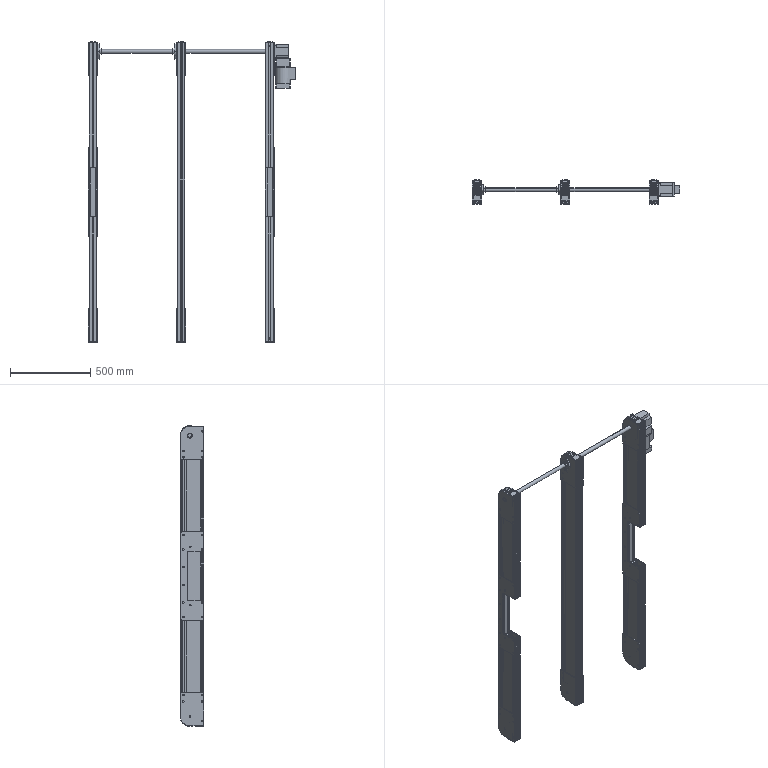Part | SolidWorks | features ReferencePattern 23, LocalLPattern 6, CompositeCurve 3 | 81 solids | 5384 faces | volume 15158359 mm3 | cylinder 2526 | plane 1758 | torus 672 | sphere 360 | cone 68 | commonest cylinder face diameters 1.2 x519 1.6 x516 9 x228 112.74 x216 20 x74 6 x53